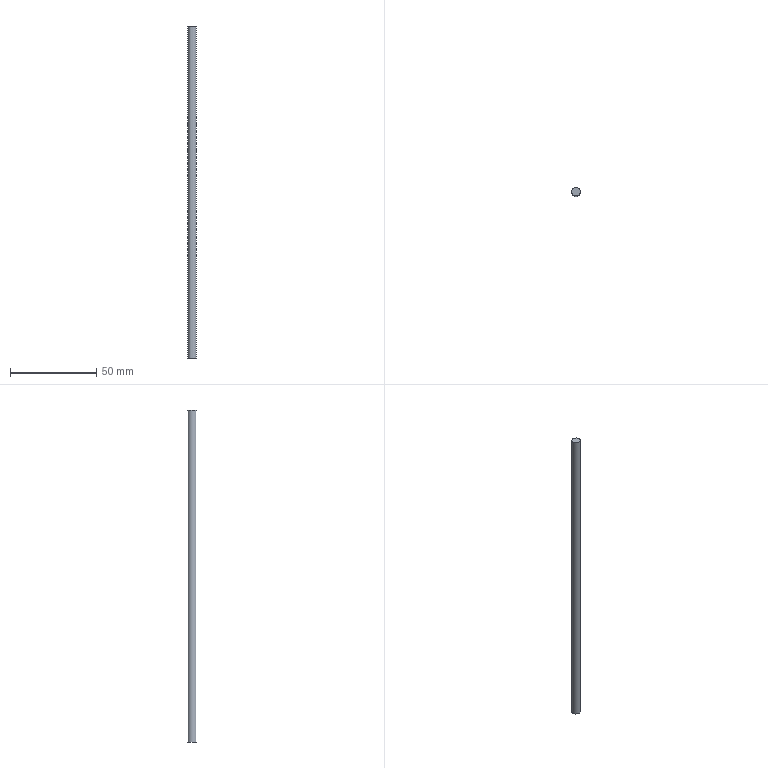Part | STEP file | gslz 2016.10.28-13_id306_x_t | 1 solid | 3 faces | box 5 x 5 x 192.275 mm | volume 3775 mm3 | plane 2 | cylinder 1 | commonest cylinder face diameters 5 x1
STEP:
#1=CARTESIAN_POINT('',(0.,0.,0.));
#2=DIRECTION('',(0.,0.,1.));
#3=DIRECTION('',(1.,0.,0.));
#4=AXIS2_PLACEMENT_3D('',#1,#2,#3);
#5=CARTESIAN_POINT('',(-249.439,153.127,73.));
#6=VERTEX_POINT('',#5);
#7=CARTESIAN_POINT('',(-251.939,153.127,73.));
#8=DIRECTION('',(0.,0.,1.));
#9=DIRECTION('',(1.,0.,0.));
#10=AXIS2_PLACEMENT_3D('',#7,#8,#9);
#11=CIRCLE('',#10,2.5);
#12=CARTESIAN_POINT('',(-251.939,153.127,80.725));
#13=DIRECTION('',(0.,0.,-1.));
#14=DIRECTION('',(0.,1.,0.));
#15=AXIS2_PLACEMENT_3D('',#12,#13,#14);
#16=CYLINDRICAL_SURFACE('',#15,2.5);
#17=CARTESIAN_POINT('',(7.854,7.725));
#18=DIRECTION('',(-1.,0.));
#19=VECTOR('',#18,1.);
#20=LINE('',#17,#19);
#21=(GEOMETRIC_REPRESENTATION_CONTEXT(2)PARAMETRIC_REPRESENTATION_CONTEXT()REPRESENTATION_CONTEXT('',''));
#22=DEFINITIONAL_REPRESENTATION('',(#20),#21);
#23=PCURVE('',#16,#22);
#24=CARTESIAN_POINT('',(-1520.,950.,73.));
#25=DIRECTION('',(0.,0.,1.));
#26=DIRECTION('',(1.,0.,0.));
#27=AXIS2_PLACEMENT_3D('',#24,#25,#26);
#28=PLANE('',#27);
#29=CARTESIAN_POINT('',(1268.061,-796.873));
#30=DIRECTION('',(1.,0.));
#31=AXIS2_PLACEMENT_2D('',#29,#30);
#32=CIRCLE('',#31,2.5);
#33=(GEOMETRIC_REPRESENTATION_CONTEXT(2)PARAMETRIC_REPRESENTATION_CONTEXT()REPRESENTATION_CONTEXT('',''));
#34=DEFINITIONAL_REPRESENTATION('',(#32),#33);
#35=PCURVE('',#28,#34);
#36=SURFACE_CURVE('',#11,(#23,#35),.PCURVE_S1.);
#37=EDGE_CURVE('',#6,#6,#36,.T.);
#38=ORIENTED_EDGE('',*,*,#37,.F.);
#39=CARTESIAN_POINT('',(-249.439,153.127,-119.275));
#40=VERTEX_POINT('',#39);
#41=CARTESIAN_POINT('',(-249.439,153.127,73.));
#42=CARTESIAN_POINT('',(-249.439,153.127,-119.275));
#43=B_SPLINE_CURVE_WITH_KNOTS('',1,(#41,#42),.UNSPECIFIED.,.F.,.F.,(2,2),(7.725,200.),.PIECEWISE_BEZIER_KNOTS.);
#44=CARTESIAN_POINT('',(7.854,0.));
#45=DIRECTION('',(0.,1.));
#46=VECTOR('',#45,1.);
#47=LINE('',#44,#46);
#48=(GEOMETRIC_REPRESENTATION_CONTEXT(2)PARAMETRIC_REPRESENTATION_CONTEXT()REPRESENTATION_CONTEXT('',''));
#49=DEFINITIONAL_REPRESENTATION('',(#47),#48);
#50=PCURVE('',#16,#49);
#51=CARTESIAN_POINT('',(1.571,0.));
#52=DIRECTION('',(0.,1.));
#53=VECTOR('',#52,1.);
#54=LINE('',#51,#53);
#55=(GEOMETRIC_REPRESENTATION_CONTEXT(2)PARAMETRIC_REPRESENTATION_CONTEXT()REPRESENTATION_CONTEXT('',''));
#56=DEFINITIONAL_REPRESENTATION('',(#54),#55);
#57=PCURVE('',#16,#56);
#58=SEAM_CURVE('',#43,(#50,#57),.PCURVE_S1.);
#59=EDGE_CURVE('',#6,#40,#58,.T.);
#60=ORIENTED_EDGE('',*,*,#59,.T.);
#61=CARTESIAN_POINT('',(-251.939,153.127,-119.275));
#62=DIRECTION('',(0.,0.,1.));
#63=DIRECTION('',(1.,0.,0.));
#64=AXIS2_PLACEMENT_3D('',#61,#62,#63);
#65=CIRCLE('',#64,2.5);
#66=CARTESIAN_POINT('',(7.854,200.));
#67=DIRECTION('',(-1.,0.));
#68=VECTOR('',#67,1.);
#69=LINE('',#66,#68);
#70=(GEOMETRIC_REPRESENTATION_CONTEXT(2)PARAMETRIC_REPRESENTATION_CONTEXT()REPRESENTATION_CONTEXT('',''));
#71=DEFINITIONAL_REPRESENTATION('',(#69),#70);
#72=PCURVE('',#16,#71);
#73=CARTESIAN_POINT('',(-251.939,153.127,-119.275));
#74=DIRECTION('',(0.,0.,1.));
#75=DIRECTION('',(1.,0.,0.));
#76=AXIS2_PLACEMENT_3D('',#73,#74,#75);
#77=PLANE('',#76);
#78=CARTESIAN_POINT('',(0.,0.));
#79=DIRECTION('',(1.,0.));
#80=AXIS2_PLACEMENT_2D('',#78,#79);
#81=CIRCLE('',#80,2.5);
#82=(GEOMETRIC_REPRESENTATION_CONTEXT(2)PARAMETRIC_REPRESENTATION_CONTEXT()REPRESENTATION_CONTEXT('',''));
#83=DEFINITIONAL_REPRESENTATION('',(#81),#82);
#84=PCURVE('',#77,#83);
#85=SURFACE_CURVE('',#65,(#72,#84),.PCURVE_S1.);
#86=EDGE_CURVE('',#40,#40,#85,.T.);
#87=ORIENTED_EDGE('',*,*,#86,.T.);
#88=ORIENTED_EDGE('',*,*,#59,.F.);
#89=EDGE_LOOP('',(#38,#60,#87,#88));
#90=FACE_BOUND('',#89,.T.);
#91=ADVANCED_FACE('',(#90),#16,.T.);
#92=ORIENTED_EDGE('',*,*,#37,.T.);
#93=EDGE_LOOP('',(#92));
#94=FACE_BOUND('',#93,.T.);
#95=ADVANCED_FACE('',(#94),#28,.T.);
#96=ORIENTED_EDGE('',*,*,#86,.F.);
#97=EDGE_LOOP('',(#96));
#98=FACE_BOUND('',#97,.T.);
#99=ADVANCED_FACE('',(#98),#77,.F.);
#100=CLOSED_SHELL('',(#91,#95,#99));
#101=MANIFOLD_SOLID_BREP('',#100);
#102=(LENGTH_UNIT()NAMED_UNIT(*)SI_UNIT(.MILLI.,.METRE.));
#103=UNCERTAINTY_MEASURE_WITH_UNIT(LENGTH_MEASURE(0.00001),#102,'','');
#104=(NAMED_UNIT(*)PLANE_ANGLE_UNIT()SI_UNIT($,.RADIAN.));
#105=(NAMED_UNIT(*)SI_UNIT($,.STERADIAN.)SOLID_ANGLE_UNIT());
#106=(GEOMETRIC_REPRESENTATION_CONTEXT(3)GLOBAL_UNCERTAINTY_ASSIGNED_CONTEXT((#103))GLOBAL_UNIT_ASSIGNED_CONTEXT((#102,#104,#105))REPRESENTATION_CONTEXT('',''));
#107=ADVANCED_BREP_SHAPE_REPRESENTATION('',(#4,#101),#106);